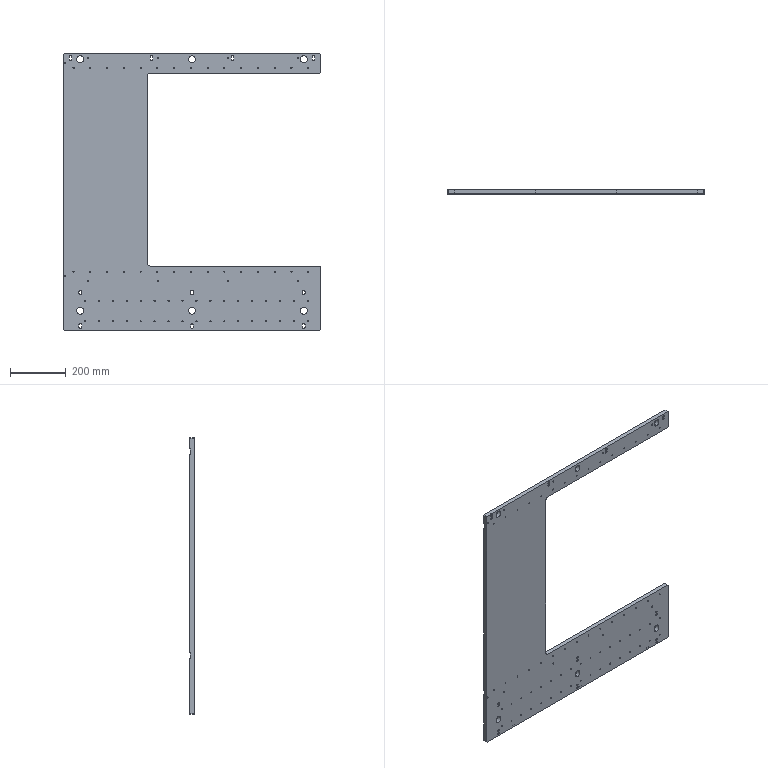Part | NX | features BREP 1 | 1 solid | 320 faces | box 920 x 15 x 990 mm | volume 7077139 mm3 | cylinder 234 | plane 74 | cone 12 | commonest cylinder face diameters 4.2 x148 15 x30 9 x18 3.3 x12 10 x12 25 x12